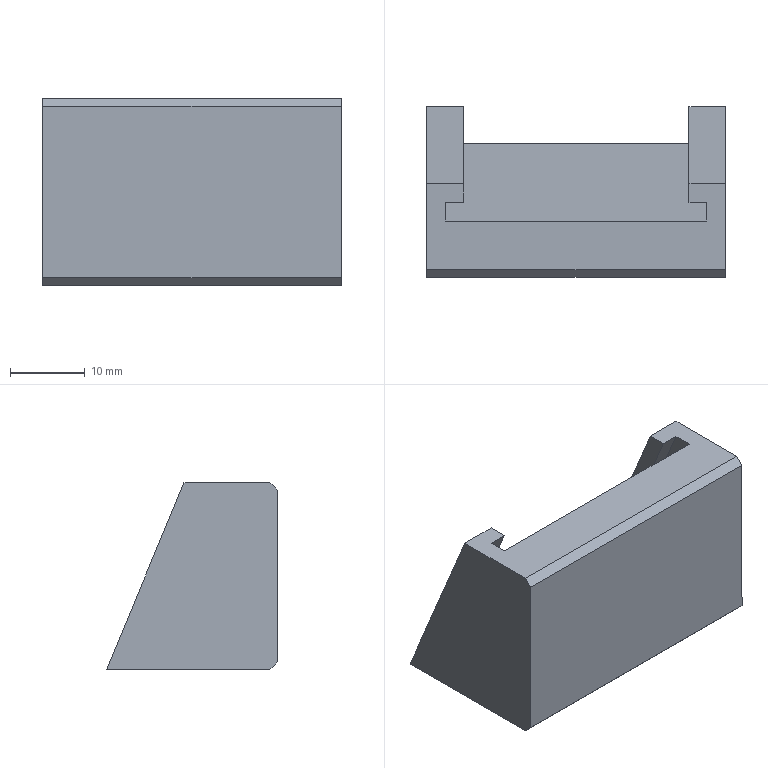Part | NX | features DATUM_CSYS 3, EXTRUDE 2, SKETCH 2 | 1 solid | 16 faces | box 40 x 22.855 x 25 mm | volume 13567 mm3 | plane 16
STEP:
#1=CARTESIAN_POINT('',(-4.874,22.855,-25.));
#2=VERTEX_POINT('',#1);
#3=CARTESIAN_POINT('',(0.,22.855,-25.));
#4=VERTEX_POINT('',#3);
#5=CARTESIAN_POINT('',(-40.,22.855,-25.));
#6=DIRECTION('',(1.,0.,0.));
#7=VECTOR('',#6,1000.);
#8=LINE('',#5,#7);
#9=EDGE_CURVE('',#2,#4,#8,.T.);
#10=ORIENTED_EDGE('',*,*,#9,.F.);
#11=CARTESIAN_POINT('',(-4.874,12.5,0.));
#12=VERTEX_POINT('',#11);
#13=CARTESIAN_POINT('',(-4.874,27.807,-36.955));
#14=DIRECTION('',(0.,-0.3827,0.9239));
#15=VECTOR('',#14,1000.);
#16=LINE('',#13,#15);
#17=EDGE_CURVE('',#2,#12,#16,.T.);
#18=ORIENTED_EDGE('',*,*,#17,.T.);
#19=CARTESIAN_POINT('',(0.,12.5,0.));
#20=VERTEX_POINT('',#19);
#21=CARTESIAN_POINT('',(-40.,12.5,0.));
#22=DIRECTION('',(1.,0.,0.));
#23=VECTOR('',#22,1000.);
#24=LINE('',#21,#23);
#25=EDGE_CURVE('',#12,#20,#24,.T.);
#26=ORIENTED_EDGE('',*,*,#25,.T.);
#27=CARTESIAN_POINT('',(0.,22.855,-25.));
#28=DIRECTION('',(0.,-0.3827,0.9239));
#29=VECTOR('',#28,1000.);
#30=LINE('',#27,#29);
#31=EDGE_CURVE('',#4,#20,#30,.T.);
#32=ORIENTED_EDGE('',*,*,#31,.F.);
#33=EDGE_LOOP('',(#10,#18,#26,#32));
#34=FACE_BOUND('',#33,.T.);
#35=CARTESIAN_POINT('',(-40.,22.855,-25.));
#36=DIRECTION('',(0.,0.9239,0.3827));
#37=DIRECTION('',(0.,-0.3827,0.9239));
#38=AXIS2_PLACEMENT_3D('',#35,#36,#37);
#39=PLANE('',#38);
#40=ADVANCED_FACE('',(#34),#39,.T.);
#41=CARTESIAN_POINT('',(0.,0.,-1.));
#42=VERTEX_POINT('',#41);
#43=CARTESIAN_POINT('',(0.,0.,-24.));
#44=VERTEX_POINT('',#43);
#45=CARTESIAN_POINT('',(0.,0.,-1.));
#46=DIRECTION('',(0.,0.,-1.));
#47=VECTOR('',#46,1000.);
#48=LINE('',#45,#47);
#49=EDGE_CURVE('',#42,#44,#48,.T.);
#50=ORIENTED_EDGE('',*,*,#49,.F.);
#51=CARTESIAN_POINT('',(-40.,0.,-1.));
#52=VERTEX_POINT('',#51);
#53=CARTESIAN_POINT('',(-40.,0.,-1.));
#54=DIRECTION('',(1.,0.,0.));
#55=VECTOR('',#54,1000.);
#56=LINE('',#53,#55);
#57=EDGE_CURVE('',#52,#42,#56,.T.);
#58=ORIENTED_EDGE('',*,*,#57,.F.);
#59=CARTESIAN_POINT('',(-40.,0.,-24.));
#60=VERTEX_POINT('',#59);
#61=CARTESIAN_POINT('',(-40.,0.,-1.));
#62=DIRECTION('',(0.,0.,-1.));
#63=VECTOR('',#62,1000.);
#64=LINE('',#61,#63);
#65=EDGE_CURVE('',#52,#60,#64,.T.);
#66=ORIENTED_EDGE('',*,*,#65,.T.);
#67=CARTESIAN_POINT('',(-40.,0.,-24.));
#68=DIRECTION('',(1.,0.,0.));
#69=VECTOR('',#68,1000.);
#70=LINE('',#67,#69);
#71=EDGE_CURVE('',#60,#44,#70,.T.);
#72=ORIENTED_EDGE('',*,*,#71,.T.);
#73=EDGE_LOOP('',(#50,#58,#66,#72));
#74=FACE_BOUND('',#73,.T.);
#75=CARTESIAN_POINT('',(-40.,0.,-1.));
#76=DIRECTION('',(0.,-1.,0.));
#77=DIRECTION('',(0.,0.,-1.));
#78=AXIS2_PLACEMENT_3D('',#75,#76,#77);
#79=PLANE('',#78);
#80=ADVANCED_FACE('',(#74),#79,.T.);
#81=CARTESIAN_POINT('',(0.,1.,-25.));
#82=VERTEX_POINT('',#81);
#83=CARTESIAN_POINT('',(0.,0.,-24.));
#84=DIRECTION('',(0.,0.7071,-0.7071));
#85=VECTOR('',#84,1000.);
#86=LINE('',#83,#85);
#87=EDGE_CURVE('',#44,#82,#86,.T.);
#88=ORIENTED_EDGE('',*,*,#87,.F.);
#89=ORIENTED_EDGE('',*,*,#71,.F.);
#90=CARTESIAN_POINT('',(-40.,1.,-25.));
#91=VERTEX_POINT('',#90);
#92=CARTESIAN_POINT('',(-40.,0.,-24.));
#93=DIRECTION('',(0.,0.7071,-0.7071));
#94=VECTOR('',#93,1000.);
#95=LINE('',#92,#94);
#96=EDGE_CURVE('',#60,#91,#95,.T.);
#97=ORIENTED_EDGE('',*,*,#96,.T.);
#98=CARTESIAN_POINT('',(-40.,1.,-25.));
#99=DIRECTION('',(1.,0.,0.));
#100=VECTOR('',#99,1000.);
#101=LINE('',#98,#100);
#102=EDGE_CURVE('',#91,#82,#101,.T.);
#103=ORIENTED_EDGE('',*,*,#102,.T.);
#104=EDGE_LOOP('',(#88,#89,#97,#103));
#105=FACE_BOUND('',#104,.T.);
#106=CARTESIAN_POINT('',(-40.,0.,-24.));
#107=DIRECTION('',(0.,-0.7071,-0.7071));
#108=DIRECTION('',(0.,0.7071,-0.7071));
#109=AXIS2_PLACEMENT_3D('',#106,#107,#108);
#110=PLANE('',#109);
#111=ADVANCED_FACE('',(#105),#110,.T.);
#112=CARTESIAN_POINT('',(-4.874,20.355,-25.));
#113=VERTEX_POINT('',#112);
#114=CARTESIAN_POINT('',(-4.874,1.,-25.));
#115=DIRECTION('',(0.,-1.,0.));
#116=VECTOR('',#115,1000.);
#117=LINE('',#114,#116);
#118=EDGE_CURVE('',#2,#113,#117,.T.);
#119=ORIENTED_EDGE('',*,*,#118,.F.);
#120=ORIENTED_EDGE('',*,*,#9,.T.);
#121=CARTESIAN_POINT('',(0.,1.,-25.));
#122=DIRECTION('',(0.,1.,0.));
#123=VECTOR('',#122,1000.);
#124=LINE('',#121,#123);
#125=EDGE_CURVE('',#82,#4,#124,.T.);
#126=ORIENTED_EDGE('',*,*,#125,.F.);
#127=ORIENTED_EDGE('',*,*,#102,.F.);
#128=CARTESIAN_POINT('',(-40.,22.855,-25.));
#129=VERTEX_POINT('',#128);
#130=CARTESIAN_POINT('',(-40.,1.,-25.));
#131=DIRECTION('',(0.,1.,0.));
#132=VECTOR('',#131,1000.);
#133=LINE('',#130,#132);
#134=EDGE_CURVE('',#91,#129,#133,.T.);
#135=ORIENTED_EDGE('',*,*,#134,.T.);
#136=CARTESIAN_POINT('',(-35.,22.855,-25.));
#137=VERTEX_POINT('',#136);
#138=CARTESIAN_POINT('',(-40.,22.855,-25.));
#139=DIRECTION('',(1.,0.,0.));
#140=VECTOR('',#139,1000.);
#141=LINE('',#138,#140);
#142=EDGE_CURVE('',#129,#137,#141,.T.);
#143=ORIENTED_EDGE('',*,*,#142,.T.);
#144=CARTESIAN_POINT('',(-35.,20.355,-25.));
#145=VERTEX_POINT('',#144);
#146=CARTESIAN_POINT('',(-35.,1.,-25.));
#147=DIRECTION('',(0.,1.,0.));
#148=VECTOR('',#147,1000.);
#149=LINE('',#146,#148);
#150=EDGE_CURVE('',#145,#137,#149,.T.);
#151=ORIENTED_EDGE('',*,*,#150,.F.);
#152=CARTESIAN_POINT('',(-37.5,20.355,-25.));
#153=VERTEX_POINT('',#152);
#154=CARTESIAN_POINT('',(-40.,20.355,-25.));
#155=DIRECTION('',(1.,0.,0.));
#156=VECTOR('',#155,1000.);
#157=LINE('',#154,#156);
#158=EDGE_CURVE('',#153,#145,#157,.T.);
#159=ORIENTED_EDGE('',*,*,#158,.F.);
#160=CARTESIAN_POINT('',(-37.5,17.855,-25.));
#161=VERTEX_POINT('',#160);
#162=CARTESIAN_POINT('',(-37.5,1.,-25.));
#163=DIRECTION('',(0.,1.,0.));
#164=VECTOR('',#163,1000.);
#165=LINE('',#162,#164);
#166=EDGE_CURVE('',#161,#153,#165,.T.);
#167=ORIENTED_EDGE('',*,*,#166,.F.);
#168=CARTESIAN_POINT('',(-2.5,17.855,-25.));
#169=VERTEX_POINT('',#168);
#170=CARTESIAN_POINT('',(-40.,17.855,-25.));
#171=DIRECTION('',(-1.,0.,0.));
#172=VECTOR('',#171,1000.);
#173=LINE('',#170,#172);
#174=EDGE_CURVE('',#169,#161,#173,.T.);
#175=ORIENTED_EDGE('',*,*,#174,.F.);
#176=CARTESIAN_POINT('',(-2.5,20.355,-25.));
#177=VERTEX_POINT('',#176);
#178=CARTESIAN_POINT('',(-2.5,1.,-25.));
#179=DIRECTION('',(0.,-1.,0.));
#180=VECTOR('',#179,1000.);
#181=LINE('',#178,#180);
#182=EDGE_CURVE('',#177,#169,#181,.T.);
#183=ORIENTED_EDGE('',*,*,#182,.F.);
#184=CARTESIAN_POINT('',(-40.,20.355,-25.));
#185=DIRECTION('',(1.,0.,0.));
#186=VECTOR('',#185,1000.);
#187=LINE('',#184,#186);
#188=EDGE_CURVE('',#113,#177,#187,.T.);
#189=ORIENTED_EDGE('',*,*,#188,.F.);
#190=EDGE_LOOP('',(#119,#120,#126,#127,#135,#143,#151,#159,#167,#175,#183,#189));
#191=FACE_BOUND('',#190,.T.);
#192=CARTESIAN_POINT('',(-40.,1.,-25.));
#193=DIRECTION('',(0.,0.,-1.));
#194=DIRECTION('',(-1.,0.,0.));
#195=AXIS2_PLACEMENT_3D('',#192,#193,#194);
#196=PLANE('',#195);
#197=ADVANCED_FACE('',(#191),#196,.T.);
#198=CARTESIAN_POINT('',(-35.,12.5,0.));
#199=VERTEX_POINT('',#198);
#200=CARTESIAN_POINT('',(-35.,27.807,-36.955));
#201=DIRECTION('',(0.,-0.3827,0.9239));
#202=VECTOR('',#201,1000.);
#203=LINE('',#200,#202);
#204=EDGE_CURVE('',#137,#199,#203,.T.);
#205=ORIENTED_EDGE('',*,*,#204,.F.);
#206=ORIENTED_EDGE('',*,*,#142,.F.);
#207=CARTESIAN_POINT('',(-40.,12.5,0.));
#208=VERTEX_POINT('',#207);
#209=CARTESIAN_POINT('',(-40.,22.855,-25.));
#210=DIRECTION('',(0.,-0.3827,0.9239));
#211=VECTOR('',#210,1000.);
#212=LINE('',#209,#211);
#213=EDGE_CURVE('',#129,#208,#212,.T.);
#214=ORIENTED_EDGE('',*,*,#213,.T.);
#215=CARTESIAN_POINT('',(-40.,12.5,0.));
#216=DIRECTION('',(1.,0.,0.));
#217=VECTOR('',#216,1000.);
#218=LINE('',#215,#217);
#219=EDGE_CURVE('',#208,#199,#218,.T.);
#220=ORIENTED_EDGE('',*,*,#219,.T.);
#221=EDGE_LOOP('',(#205,#206,#214,#220));
#222=FACE_BOUND('',#221,.T.);
#223=CARTESIAN_POINT('',(-40.,22.855,-25.));
#224=DIRECTION('',(0.,0.9239,0.3827));
#225=DIRECTION('',(0.,-0.3827,0.9239));
#226=AXIS2_PLACEMENT_3D('',#223,#224,#225);
#227=PLANE('',#226);
#228=ADVANCED_FACE('',(#222),#227,.T.);
#229=CARTESIAN_POINT('',(-35.,10.,0.));
#230=VERTEX_POINT('',#229);
#231=CARTESIAN_POINT('',(-35.,12.5,0.));
#232=DIRECTION('',(0.,-1.,0.));
#233=VECTOR('',#232,1000.);
#234=LINE('',#231,#233);
#235=EDGE_CURVE('',#199,#230,#234,.T.);
#236=ORIENTED_EDGE('',*,*,#235,.F.);
#237=ORIENTED_EDGE('',*,*,#219,.F.);
#238=CARTESIAN_POINT('',(-40.,1.,0.));
#239=VERTEX_POINT('',#238);
#240=CARTESIAN_POINT('',(-40.,12.5,0.));
#241=DIRECTION('',(0.,-1.,0.));
#242=VECTOR('',#241,1000.);
#243=LINE('',#240,#242);
#244=EDGE_CURVE('',#208,#239,#243,.T.);
#245=ORIENTED_EDGE('',*,*,#244,.T.);
#246=CARTESIAN_POINT('',(0.,1.,0.));
#247=VERTEX_POINT('',#246);
#248=CARTESIAN_POINT('',(-40.,1.,0.));
#249=DIRECTION('',(1.,0.,0.));
#250=VECTOR('',#249,1000.);
#251=LINE('',#248,#250);
#252=EDGE_CURVE('',#239,#247,#251,.T.);
#253=ORIENTED_EDGE('',*,*,#252,.T.);
#254=CARTESIAN_POINT('',(0.,12.5,0.));
#255=DIRECTION('',(0.,-1.,0.));
#256=VECTOR('',#255,1000.);
#257=LINE('',#254,#256);
#258=EDGE_CURVE('',#20,#247,#257,.T.);
#259=ORIENTED_EDGE('',*,*,#258,.F.);
#260=ORIENTED_EDGE('',*,*,#25,.F.);
#261=CARTESIAN_POINT('',(-4.874,10.,0.));
#262=VERTEX_POINT('',#261);
#263=CARTESIAN_POINT('',(-4.874,10.,0.));
#264=DIRECTION('',(0.,1.,0.));
#265=VECTOR('',#264,1000.);
#266=LINE('',#263,#265);
#267=EDGE_CURVE('',#262,#12,#266,.T.);
#268=ORIENTED_EDGE('',*,*,#267,.F.);
#269=CARTESIAN_POINT('',(-2.5,10.,0.));
#270=VERTEX_POINT('',#269);
#271=CARTESIAN_POINT('',(-2.5,10.,0.));
#272=DIRECTION('',(-1.,0.,0.));
#273=VECTOR('',#272,1000.);
#274=LINE('',#271,#273);
#275=EDGE_CURVE('',#270,#262,#274,.T.);
#276=ORIENTED_EDGE('',*,*,#275,.F.);
#277=CARTESIAN_POINT('',(-2.5,7.5,0.));
#278=VERTEX_POINT('',#277);
#279=CARTESIAN_POINT('',(-2.5,7.5,0.));
#280=DIRECTION('',(0.,1.,0.));
#281=VECTOR('',#280,1000.);
#282=LINE('',#279,#281);
#283=EDGE_CURVE('',#278,#270,#282,.T.);
#284=ORIENTED_EDGE('',*,*,#283,.F.);
#285=CARTESIAN_POINT('',(-37.5,7.5,0.));
#286=VERTEX_POINT('',#285);
#287=CARTESIAN_POINT('',(-20.,7.5,0.));
#288=DIRECTION('',(1.,0.,0.));
#289=VECTOR('',#288,1000.);
#290=LINE('',#287,#289);
#291=EDGE_CURVE('',#286,#278,#290,.T.);
#292=ORIENTED_EDGE('',*,*,#291,.F.);
#293=CARTESIAN_POINT('',(-37.5,10.,0.));
#294=VERTEX_POINT('',#293);
#295=CARTESIAN_POINT('',(-37.5,10.,0.));
#296=DIRECTION('',(0.,-1.,0.));
#297=VECTOR('',#296,1000.);
#298=LINE('',#295,#297);
#299=EDGE_CURVE('',#294,#286,#298,.T.);
#300=ORIENTED_EDGE('',*,*,#299,.F.);
#301=CARTESIAN_POINT('',(-35.,10.,0.));
#302=DIRECTION('',(-1.,0.,0.));
#303=VECTOR('',#302,1000.);
#304=LINE('',#301,#303);
#305=EDGE_CURVE('',#230,#294,#304,.T.);
#306=ORIENTED_EDGE('',*,*,#305,.F.);
#307=EDGE_LOOP('',(#236,#237,#245,#253,#259,#260,#268,#276,#284,#292,#300,#306));
#308=FACE_BOUND('',#307,.T.);
#309=CARTESIAN_POINT('',(-40.,12.5,0.));
#310=DIRECTION('',(0.,0.,1.));
#311=DIRECTION('',(1.,0.,0.));
#312=AXIS2_PLACEMENT_3D('',#309,#310,#311);
#313=PLANE('',#312);
#314=ADVANCED_FACE('',(#308),#313,.T.);
#315=CARTESIAN_POINT('',(0.,1.,0.));
#316=DIRECTION('',(0.,-0.7071,-0.7071));
#317=VECTOR('',#316,1000.);
#318=LINE('',#315,#317);
#319=EDGE_CURVE('',#247,#42,#318,.T.);
#320=ORIENTED_EDGE('',*,*,#319,.F.);
#321=ORIENTED_EDGE('',*,*,#252,.F.);
#322=CARTESIAN_POINT('',(-40.,1.,0.));
#323=DIRECTION('',(0.,-0.7071,-0.7071));
#324=VECTOR('',#323,1000.);
#325=LINE('',#322,#324);
#326=EDGE_CURVE('',#239,#52,#325,.T.);
#327=ORIENTED_EDGE('',*,*,#326,.T.);
#328=ORIENTED_EDGE('',*,*,#57,.T.);
#329=EDGE_LOOP('',(#320,#321,#327,#328));
#330=FACE_BOUND('',#329,.T.);
#331=CARTESIAN_POINT('',(-40.,1.,0.));
#332=DIRECTION('',(0.,-0.7071,0.7071));
#333=DIRECTION('',(0.,-0.7071,-0.7071));
#334=AXIS2_PLACEMENT_3D('',#331,#332,#333);
#335=PLANE('',#334);
#336=ADVANCED_FACE('',(#330),#335,.T.);
#337=ORIENTED_EDGE('',*,*,#65,.F.);
#338=ORIENTED_EDGE('',*,*,#326,.F.);
#339=ORIENTED_EDGE('',*,*,#244,.F.);
#340=ORIENTED_EDGE('',*,*,#213,.F.);
#341=ORIENTED_EDGE('',*,*,#134,.F.);
#342=ORIENTED_EDGE('',*,*,#96,.F.);
#343=EDGE_LOOP('',(#337,#338,#339,#340,#341,#342));
#344=FACE_BOUND('',#343,.T.);
#345=CARTESIAN_POINT('',(-40.,0.,0.));
#346=DIRECTION('',(1.,0.,0.));
#347=DIRECTION('',(0.,0.,-1.));
#348=AXIS2_PLACEMENT_3D('',#345,#346,#347);
#349=PLANE('',#348);
#350=ADVANCED_FACE('',(#344),#349,.F.);
#351=ORIENTED_EDGE('',*,*,#49,.T.);
#352=ORIENTED_EDGE('',*,*,#87,.T.);
#353=ORIENTED_EDGE('',*,*,#125,.T.);
#354=ORIENTED_EDGE('',*,*,#31,.T.);
#355=ORIENTED_EDGE('',*,*,#258,.T.);
#356=ORIENTED_EDGE('',*,*,#319,.T.);
#357=EDGE_LOOP('',(#351,#352,#353,#354,#355,#356));
#358=FACE_BOUND('',#357,.T.);
#359=CARTESIAN_POINT('',(0.,0.,0.));
#360=DIRECTION('',(1.,0.,0.));
#361=DIRECTION('',(0.,0.,-1.));
#362=AXIS2_PLACEMENT_3D('',#359,#360,#361);
#363=PLANE('',#362);
#364=ADVANCED_FACE('',(#358),#363,.T.);
#365=ORIENTED_EDGE('',*,*,#166,.T.);
#366=CARTESIAN_POINT('',(-37.5,25.307,-36.955));
#367=DIRECTION('',(0.,-0.3827,0.9239));
#368=VECTOR('',#367,1000.);
#369=LINE('',#366,#368);
#370=EDGE_CURVE('',#294,#153,#369,.F.);
#371=ORIENTED_EDGE('',*,*,#370,.F.);
#372=ORIENTED_EDGE('',*,*,#299,.T.);
#373=CARTESIAN_POINT('',(-37.5,22.807,-36.955));
#374=DIRECTION('',(0.,-0.3827,0.9239));
#375=VECTOR('',#374,1000.);
#376=LINE('',#373,#375);
#377=EDGE_CURVE('',#286,#161,#376,.F.);
#378=ORIENTED_EDGE('',*,*,#377,.T.);
#379=EDGE_LOOP('',(#365,#371,#372,#378));
#380=FACE_BOUND('',#379,.T.);
#381=CARTESIAN_POINT('',(-37.5,25.307,-36.955));
#382=DIRECTION('',(-1.,0.,0.));
#383=DIRECTION('',(0.,0.,1.));
#384=AXIS2_PLACEMENT_3D('',#381,#382,#383);
#385=PLANE('',#384);
#386=ADVANCED_FACE('',(#380),#385,.F.);
#387=ORIENTED_EDGE('',*,*,#174,.T.);
#388=ORIENTED_EDGE('',*,*,#377,.F.);
#389=ORIENTED_EDGE('',*,*,#291,.T.);
#390=CARTESIAN_POINT('',(-2.5,22.807,-36.955));
#391=DIRECTION('',(0.,-0.3827,0.9239));
#392=VECTOR('',#391,1000.);
#393=LINE('',#390,#392);
#394=EDGE_CURVE('',#278,#169,#393,.F.);
#395=ORIENTED_EDGE('',*,*,#394,.T.);
#396=EDGE_LOOP('',(#387,#388,#389,#395));
#397=FACE_BOUND('',#396,.T.);
#398=CARTESIAN_POINT('',(-20.,22.807,-36.955));
#399=DIRECTION('',(0.,-0.9239,-0.3827));
#400=DIRECTION('',(0.,0.3827,-0.9239));
#401=AXIS2_PLACEMENT_3D('',#398,#399,#400);
#402=PLANE('',#401);
#403=ADVANCED_FACE('',(#397),#402,.F.);
#404=ORIENTED_EDGE('',*,*,#182,.T.);
#405=ORIENTED_EDGE('',*,*,#394,.F.);
#406=ORIENTED_EDGE('',*,*,#283,.T.);
#407=CARTESIAN_POINT('',(-2.5,25.307,-36.955));
#408=DIRECTION('',(0.,-0.3827,0.9239));
#409=VECTOR('',#408,1000.);
#410=LINE('',#407,#409);
#411=EDGE_CURVE('',#270,#177,#410,.F.);
#412=ORIENTED_EDGE('',*,*,#411,.T.);
#413=EDGE_LOOP('',(#404,#405,#406,#412));
#414=FACE_BOUND('',#413,.T.);
#415=CARTESIAN_POINT('',(-2.5,22.807,-36.955));
#416=DIRECTION('',(1.,0.,0.));
#417=DIRECTION('',(0.,0.,-1.));
#418=AXIS2_PLACEMENT_3D('',#415,#416,#417);
#419=PLANE('',#418);
#420=ADVANCED_FACE('',(#414),#419,.F.);
#421=ORIENTED_EDGE('',*,*,#188,.T.);
#422=ORIENTED_EDGE('',*,*,#411,.F.);
#423=ORIENTED_EDGE('',*,*,#275,.T.);
#424=CARTESIAN_POINT('',(-4.874,25.307,-36.955));
#425=DIRECTION('',(0.,-0.3827,0.9239));
#426=VECTOR('',#425,1000.);
#427=LINE('',#424,#426);
#428=EDGE_CURVE('',#262,#113,#427,.F.);
#429=ORIENTED_EDGE('',*,*,#428,.T.);
#430=EDGE_LOOP('',(#421,#422,#423,#429));
#431=FACE_BOUND('',#430,.T.);
#432=CARTESIAN_POINT('',(-2.5,25.307,-36.955));
#433=DIRECTION('',(0.,0.9239,0.3827));
#434=DIRECTION('',(0.,-0.3827,0.9239));
#435=AXIS2_PLACEMENT_3D('',#432,#433,#434);
#436=PLANE('',#435);
#437=ADVANCED_FACE('',(#431),#436,.F.);
#438=ORIENTED_EDGE('',*,*,#118,.T.);
#439=ORIENTED_EDGE('',*,*,#428,.F.);
#440=ORIENTED_EDGE('',*,*,#267,.T.);
#441=ORIENTED_EDGE('',*,*,#17,.F.);
#442=EDGE_LOOP('',(#438,#439,#440,#441));
#443=FACE_BOUND('',#442,.T.);
#444=CARTESIAN_POINT('',(-4.874,25.307,-36.955));
#445=DIRECTION('',(1.,0.,0.));
#446=DIRECTION('',(0.,1.,0.));
#447=AXIS2_PLACEMENT_3D('',#444,#445,#446);
#448=PLANE('',#447);
#449=ADVANCED_FACE('',(#443),#448,.F.);
#450=ORIENTED_EDGE('',*,*,#150,.T.);
#451=ORIENTED_EDGE('',*,*,#204,.T.);
#452=ORIENTED_EDGE('',*,*,#235,.T.);
#453=CARTESIAN_POINT('',(-35.,25.307,-36.955));
#454=DIRECTION('',(0.,-0.3827,0.9239));
#455=VECTOR('',#454,1000.);
#456=LINE('',#453,#455);
#457=EDGE_CURVE('',#230,#145,#456,.F.);
#458=ORIENTED_EDGE('',*,*,#457,.T.);
#459=EDGE_LOOP('',(#450,#451,#452,#458));
#460=FACE_BOUND('',#459,.T.);
#461=CARTESIAN_POINT('',(-35.,27.807,-36.955));
#462=DIRECTION('',(-1.,0.,0.));
#463=DIRECTION('',(0.,-1.,0.));
#464=AXIS2_PLACEMENT_3D('',#461,#462,#463);
#465=PLANE('',#464);
#466=ADVANCED_FACE('',(#460),#465,.F.);
#467=ORIENTED_EDGE('',*,*,#158,.T.);
#468=ORIENTED_EDGE('',*,*,#457,.F.);
#469=ORIENTED_EDGE('',*,*,#305,.T.);
#470=ORIENTED_EDGE('',*,*,#370,.T.);
#471=EDGE_LOOP('',(#467,#468,#469,#470));
#472=FACE_BOUND('',#471,.T.);
#473=CARTESIAN_POINT('',(-35.,25.307,-36.955));
#474=DIRECTION('',(0.,0.9239,0.3827));
#475=DIRECTION('',(0.,-0.3827,0.9239));
#476=AXIS2_PLACEMENT_3D('',#473,#474,#475);
#477=PLANE('',#476);
#478=ADVANCED_FACE('',(#472),#477,.F.);
#479=CLOSED_SHELL('',(#40,#80,#111,#197,#228,#314,#336,#350,#364,#386,#403,#420,#437,#449,#466,#478));
#480=MANIFOLD_SOLID_BREP('',#479);
#481=(LENGTH_UNIT()NAMED_UNIT(*)SI_UNIT(.MILLI.,.METRE.));
#482=UNCERTAINTY_MEASURE_WITH_UNIT(LENGTH_MEASURE(0.00001),#481,'','');
#483=(NAMED_UNIT(*)PLANE_ANGLE_UNIT()SI_UNIT($,.RADIAN.));
#484=(NAMED_UNIT(*)SI_UNIT($,.STERADIAN.)SOLID_ANGLE_UNIT());
#485=(GEOMETRIC_REPRESENTATION_CONTEXT(3)GLOBAL_UNCERTAINTY_ASSIGNED_CONTEXT((#482))GLOBAL_UNIT_ASSIGNED_CONTEXT((#481,#483,#484))REPRESENTATION_CONTEXT('',''));
#486=ADVANCED_BREP_SHAPE_REPRESENTATION('',(#480),#485);